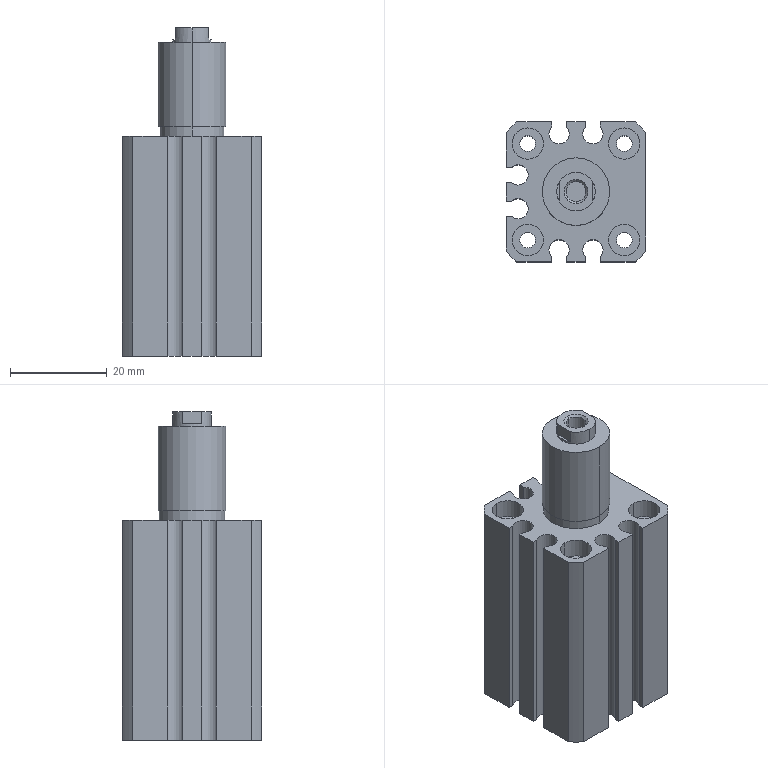Part | STEP file | ASND-0110-1 | 1 solid | 118 faces | box 29 x 29 x 68 mm | volume 33970 mm3 | cylinder 62 | plane 50 | cone 6 | commonest cylinder face diameters 3.24 x16 6.5 x16 3.5 x8 4.13 x6 4.2 x6 38 x4